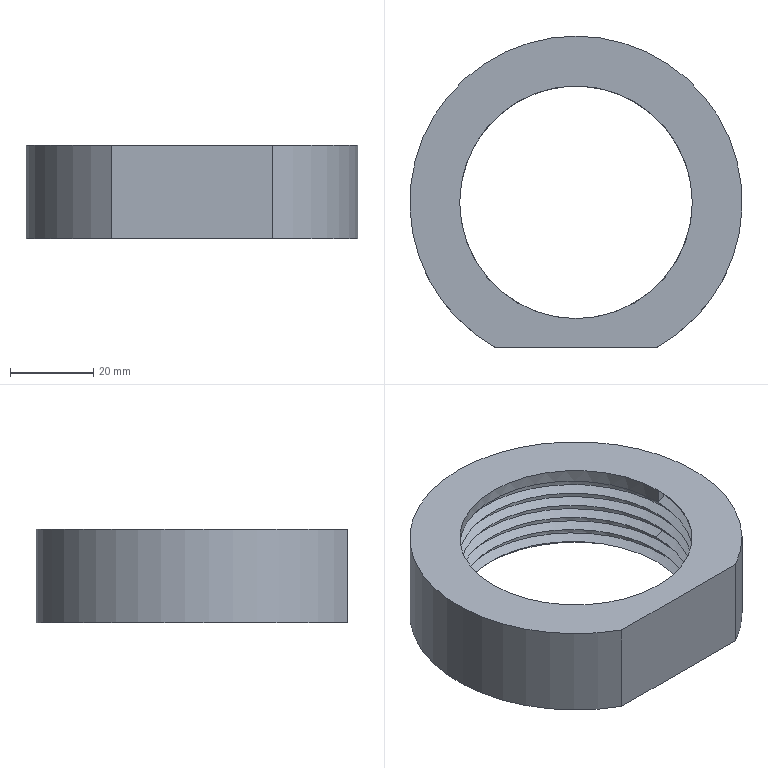Part | STEP file | SCREW-BUSH2_id542_x_t | 1 solid | 13 faces | box 80 x 75 x 22.5 mm | volume 49484 mm3 | spline 7 | plane 4 | cylinder 2 | commonest cylinder face diameters 56 x1 80 x1